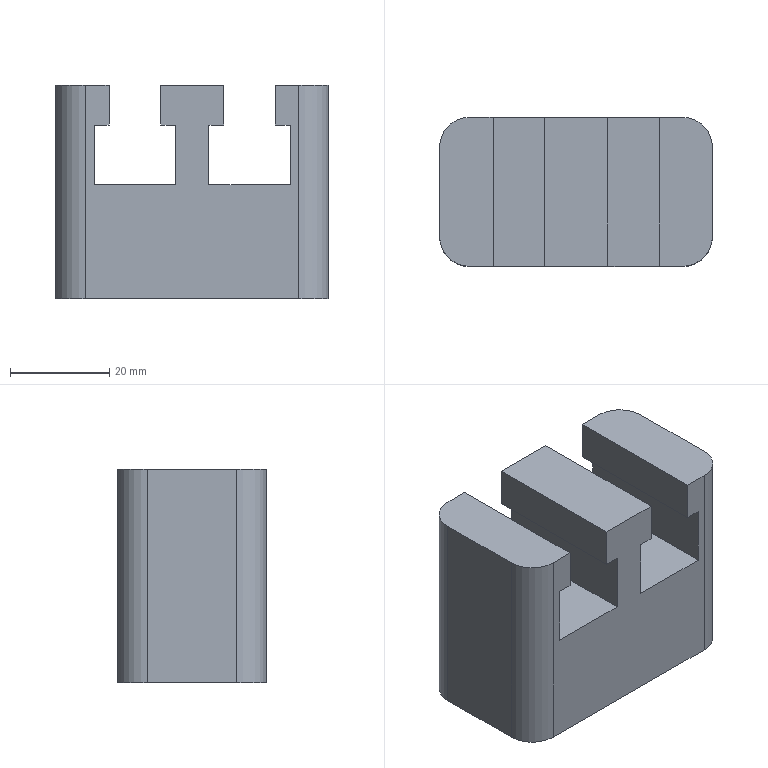Part | STEP file | solid 130 | 1 solid | 41 faces | box 55 x 30 x 43 mm | volume 51024 mm3 | plane 29 | cylinder 8 | cone 2 | other 2 | commonest cylinder face diameters 12 x4 6.7 x2 8 x2